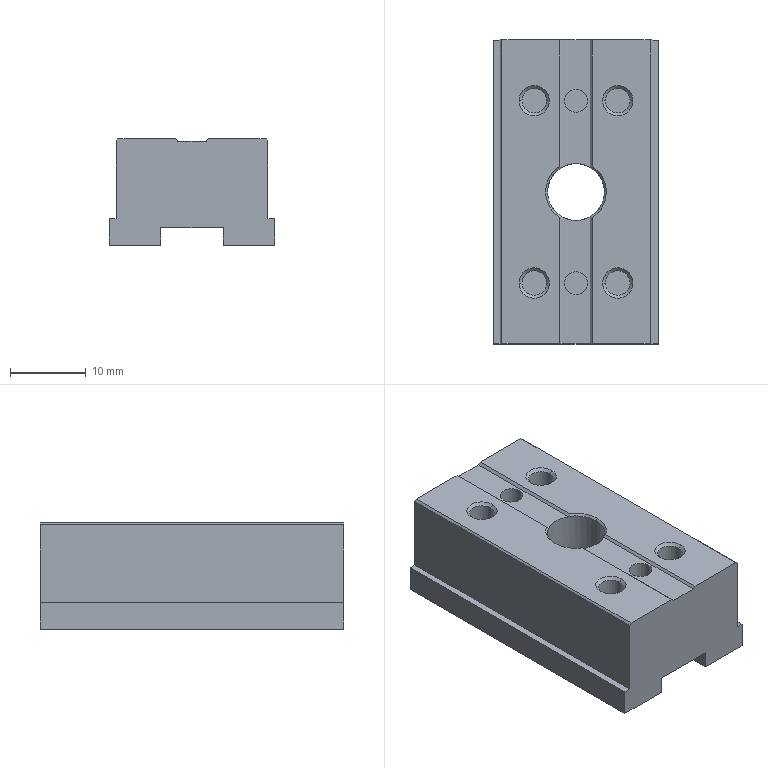Part | STEP file | 1 solid | 54 faces | box 21.8 x 40 x 14 mm | volume 9965 mm3 | plane 29 | cylinder 14 | cone 11 | commonest cylinder face diameters 3.242 x8 3.01 x4 7.5 x2